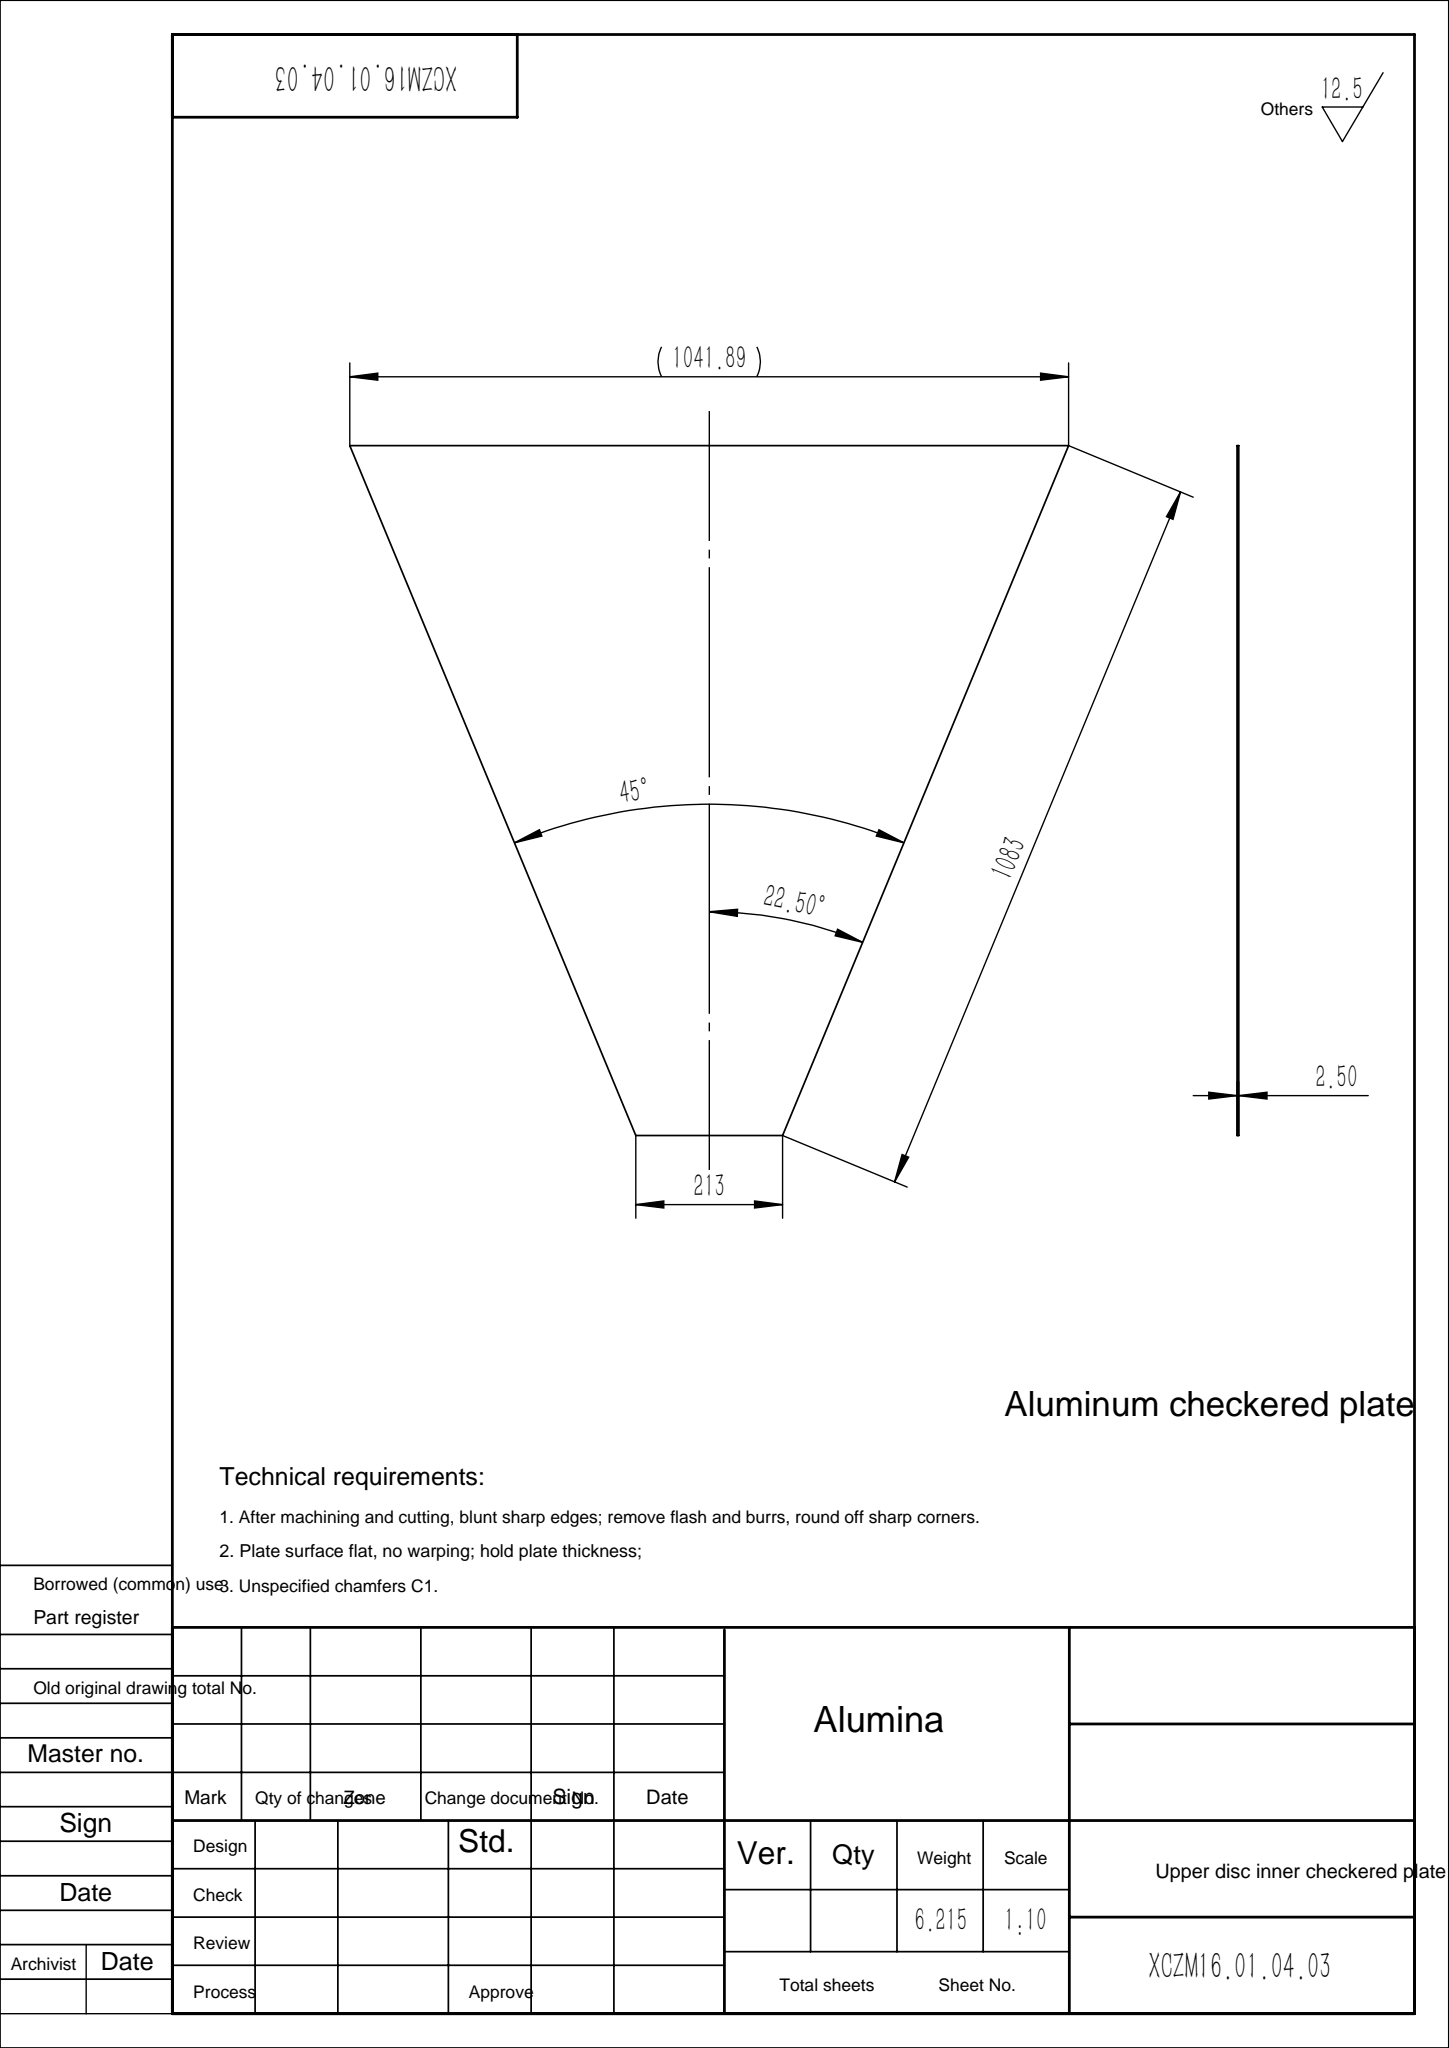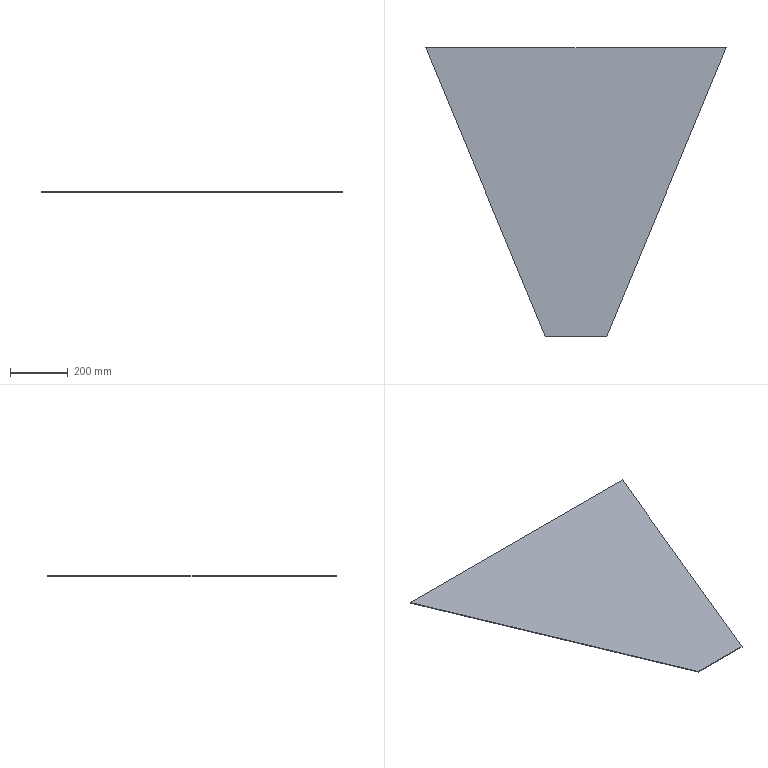Part | SolidWorks | features Extrusion 1 | 1 solid | 6 faces | box 1042 x 1001 x 2.5 mm | volume 1569496 mm3 | plane 6
STEP:
#1=CARTESIAN_POINT('',(-520.946,1000.562,0.));
#2=VERTEX_POINT('',#1);
#3=CARTESIAN_POINT('',(520.946,1000.562,0.));
#4=VERTEX_POINT('',#3);
#5=CARTESIAN_POINT('',(0.,1000.562,0.));
#6=DIRECTION('',(1.,0.,0.));
#7=VECTOR('',#6,1000.);
#8=LINE('',#5,#7);
#9=EDGE_CURVE('',#2,#4,#8,.T.);
#10=ORIENTED_EDGE('',*,*,#9,.F.);
#11=CARTESIAN_POINT('',(-520.946,1000.562,2.5));
#12=VERTEX_POINT('',#11);
#13=CARTESIAN_POINT('',(-520.946,1000.562,2.5));
#14=DIRECTION('',(0.,0.,-1.));
#15=VECTOR('',#14,1000.);
#16=LINE('',#13,#15);
#17=EDGE_CURVE('',#12,#2,#16,.T.);
#18=ORIENTED_EDGE('',*,*,#17,.F.);
#19=CARTESIAN_POINT('',(520.946,1000.562,2.5));
#20=VERTEX_POINT('',#19);
#21=CARTESIAN_POINT('',(0.,1000.562,2.5));
#22=DIRECTION('',(1.,0.,0.));
#23=VECTOR('',#22,1000.);
#24=LINE('',#21,#23);
#25=EDGE_CURVE('',#12,#20,#24,.T.);
#26=ORIENTED_EDGE('',*,*,#25,.T.);
#27=CARTESIAN_POINT('',(520.946,1000.562,2.5));
#28=DIRECTION('',(0.,0.,-1.));
#29=VECTOR('',#28,1000.);
#30=LINE('',#27,#29);
#31=EDGE_CURVE('',#20,#4,#30,.T.);
#32=ORIENTED_EDGE('',*,*,#31,.T.);
#33=EDGE_LOOP('',(#10,#18,#26,#32));
#34=FACE_OUTER_BOUND('',#33,.T.);
#35=CARTESIAN_POINT('',(0.,1000.562,2.5));
#36=DIRECTION('',(0.,1.,0.));
#37=DIRECTION('',(0.,0.,1.));
#38=AXIS2_PLACEMENT_3D('',#35,#36,#37);
#39=PLANE('',#38);
#40=ADVANCED_FACE('',(#34),#39,.T.);
#41=CARTESIAN_POINT('',(-106.5,0.,0.));
#42=VERTEX_POINT('',#41);
#43=CARTESIAN_POINT('',(-90.903,-37.653,0.));
#44=DIRECTION('',(-0.3827,0.9239,0.));
#45=VECTOR('',#44,1000.);
#46=LINE('',#43,#45);
#47=EDGE_CURVE('',#42,#2,#46,.T.);
#48=ORIENTED_EDGE('',*,*,#47,.F.);
#49=CARTESIAN_POINT('',(-106.5,0.,2.5));
#50=VERTEX_POINT('',#49);
#51=CARTESIAN_POINT('',(-106.5,0.,2.5));
#52=DIRECTION('',(0.,0.,-1.));
#53=VECTOR('',#52,1000.);
#54=LINE('',#51,#53);
#55=EDGE_CURVE('',#50,#42,#54,.T.);
#56=ORIENTED_EDGE('',*,*,#55,.F.);
#57=CARTESIAN_POINT('',(-90.903,-37.653,2.5));
#58=DIRECTION('',(-0.3827,0.9239,0.));
#59=VECTOR('',#58,1000.);
#60=LINE('',#57,#59);
#61=EDGE_CURVE('',#50,#12,#60,.T.);
#62=ORIENTED_EDGE('',*,*,#61,.T.);
#63=ORIENTED_EDGE('',*,*,#17,.T.);
#64=EDGE_LOOP('',(#48,#56,#62,#63));
#65=FACE_OUTER_BOUND('',#64,.T.);
#66=CARTESIAN_POINT('',(-90.903,-37.653,2.5));
#67=DIRECTION('',(-0.9239,-0.3827,0.));
#68=DIRECTION('',(0.3827,-0.9239,0.));
#69=AXIS2_PLACEMENT_3D('',#66,#67,#68);
#70=PLANE('',#69);
#71=ADVANCED_FACE('',(#65),#70,.T.);
#72=CARTESIAN_POINT('',(106.5,0.,0.));
#73=VERTEX_POINT('',#72);
#74=CARTESIAN_POINT('',(0.,0.,0.));
#75=DIRECTION('',(1.,0.,0.));
#76=VECTOR('',#75,1000.);
#77=LINE('',#74,#76);
#78=EDGE_CURVE('',#42,#73,#77,.T.);
#79=ORIENTED_EDGE('',*,*,#78,.T.);
#80=CARTESIAN_POINT('',(106.5,0.,2.5));
#81=VERTEX_POINT('',#80);
#82=CARTESIAN_POINT('',(106.5,0.,2.5));
#83=DIRECTION('',(0.,0.,-1.));
#84=VECTOR('',#83,1000.);
#85=LINE('',#82,#84);
#86=EDGE_CURVE('',#81,#73,#85,.T.);
#87=ORIENTED_EDGE('',*,*,#86,.F.);
#88=CARTESIAN_POINT('',(0.,0.,2.5));
#89=DIRECTION('',(1.,0.,0.));
#90=VECTOR('',#89,1000.);
#91=LINE('',#88,#90);
#92=EDGE_CURVE('',#50,#81,#91,.T.);
#93=ORIENTED_EDGE('',*,*,#92,.F.);
#94=ORIENTED_EDGE('',*,*,#55,.T.);
#95=EDGE_LOOP('',(#79,#87,#93,#94));
#96=FACE_OUTER_BOUND('',#95,.T.);
#97=CARTESIAN_POINT('',(0.,0.,2.5));
#98=DIRECTION('',(0.,1.,0.));
#99=DIRECTION('',(0.,0.,1.));
#100=AXIS2_PLACEMENT_3D('',#97,#98,#99);
#101=PLANE('',#100);
#102=ADVANCED_FACE('',(#96),#101,.F.);
#103=CARTESIAN_POINT('',(90.903,-37.653,0.));
#104=DIRECTION('',(0.3827,0.9239,0.));
#105=VECTOR('',#104,1000.);
#106=LINE('',#103,#105);
#107=EDGE_CURVE('',#73,#4,#106,.T.);
#108=ORIENTED_EDGE('',*,*,#107,.T.);
#109=ORIENTED_EDGE('',*,*,#31,.F.);
#110=CARTESIAN_POINT('',(90.903,-37.653,2.5));
#111=DIRECTION('',(0.3827,0.9239,0.));
#112=VECTOR('',#111,1000.);
#113=LINE('',#110,#112);
#114=EDGE_CURVE('',#81,#20,#113,.T.);
#115=ORIENTED_EDGE('',*,*,#114,.F.);
#116=ORIENTED_EDGE('',*,*,#86,.T.);
#117=EDGE_LOOP('',(#108,#109,#115,#116));
#118=FACE_OUTER_BOUND('',#117,.T.);
#119=CARTESIAN_POINT('',(90.903,-37.653,2.5));
#120=DIRECTION('',(-0.9239,0.3827,0.));
#121=DIRECTION('',(-0.3827,-0.9239,0.));
#122=AXIS2_PLACEMENT_3D('',#119,#120,#121);
#123=PLANE('',#122);
#124=ADVANCED_FACE('',(#118),#123,.F.);
#125=ORIENTED_EDGE('',*,*,#25,.F.);
#126=ORIENTED_EDGE('',*,*,#61,.F.);
#127=ORIENTED_EDGE('',*,*,#92,.T.);
#128=ORIENTED_EDGE('',*,*,#114,.T.);
#129=EDGE_LOOP('',(#125,#126,#127,#128));
#130=FACE_OUTER_BOUND('',#129,.T.);
#131=CARTESIAN_POINT('',(0.,0.,2.5));
#132=DIRECTION('',(0.,0.,1.));
#133=DIRECTION('',(1.,0.,0.));
#134=AXIS2_PLACEMENT_3D('',#131,#132,#133);
#135=PLANE('',#134);
#136=ADVANCED_FACE('',(#130),#135,.T.);
#137=ORIENTED_EDGE('',*,*,#9,.T.);
#138=ORIENTED_EDGE('',*,*,#107,.F.);
#139=ORIENTED_EDGE('',*,*,#78,.F.);
#140=ORIENTED_EDGE('',*,*,#47,.T.);
#141=EDGE_LOOP('',(#137,#138,#139,#140));
#142=FACE_OUTER_BOUND('',#141,.T.);
#143=CARTESIAN_POINT('',(0.,0.,0.));
#144=DIRECTION('',(0.,0.,1.));
#145=DIRECTION('',(1.,0.,0.));
#146=AXIS2_PLACEMENT_3D('',#143,#144,#145);
#147=PLANE('',#146);
#148=ADVANCED_FACE('',(#142),#147,.F.);
#149=CLOSED_SHELL('',(#40,#71,#102,#124,#136,#148));
#150=MANIFOLD_SOLID_BREP('',#149);
#151=CARTESIAN_POINT('',(0.,0.,0.));
#152=DIRECTION('',(0.,0.,1.));
#153=DIRECTION('',(1.,0.,0.));
#154=AXIS2_PLACEMENT_3D('',#151,#152,#153);
#155=(LENGTH_UNIT()NAMED_UNIT(*)SI_UNIT(.MILLI.,.METRE.));
#156=UNCERTAINTY_MEASURE_WITH_UNIT(LENGTH_MEASURE(0.00001),#155,'','');
#157=(NAMED_UNIT(*)PLANE_ANGLE_UNIT()SI_UNIT($,.RADIAN.));
#158=(NAMED_UNIT(*)SI_UNIT($,.STERADIAN.)SOLID_ANGLE_UNIT());
#159=(GEOMETRIC_REPRESENTATION_CONTEXT(3)GLOBAL_UNCERTAINTY_ASSIGNED_CONTEXT((#156))GLOBAL_UNIT_ASSIGNED_CONTEXT((#155,#157,#158))REPRESENTATION_CONTEXT('',''));
#160=ADVANCED_BREP_SHAPE_REPRESENTATION('',(#150,#154),#159);